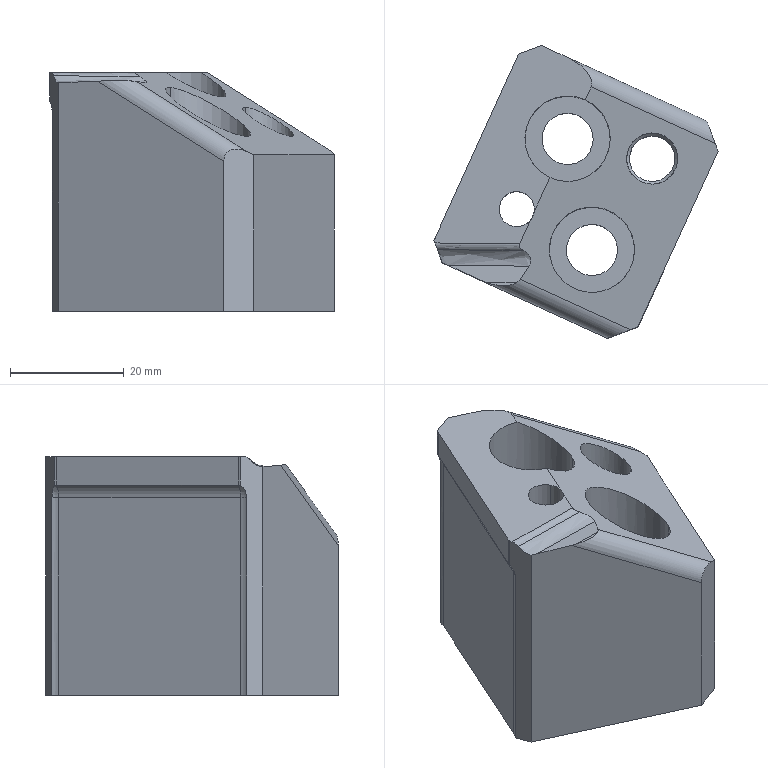Part | CATIA | 1 solid | 48 faces | box 49.997 x 51.489 x 42 mm | volume 42846 mm3 | cylinder 21 | plane 15 | spline 6 | cone 4 | other 2 | commonest cylinder face diameters 9 x6 6 x5 15 x4 6.2 x2 8 x2 13 x2